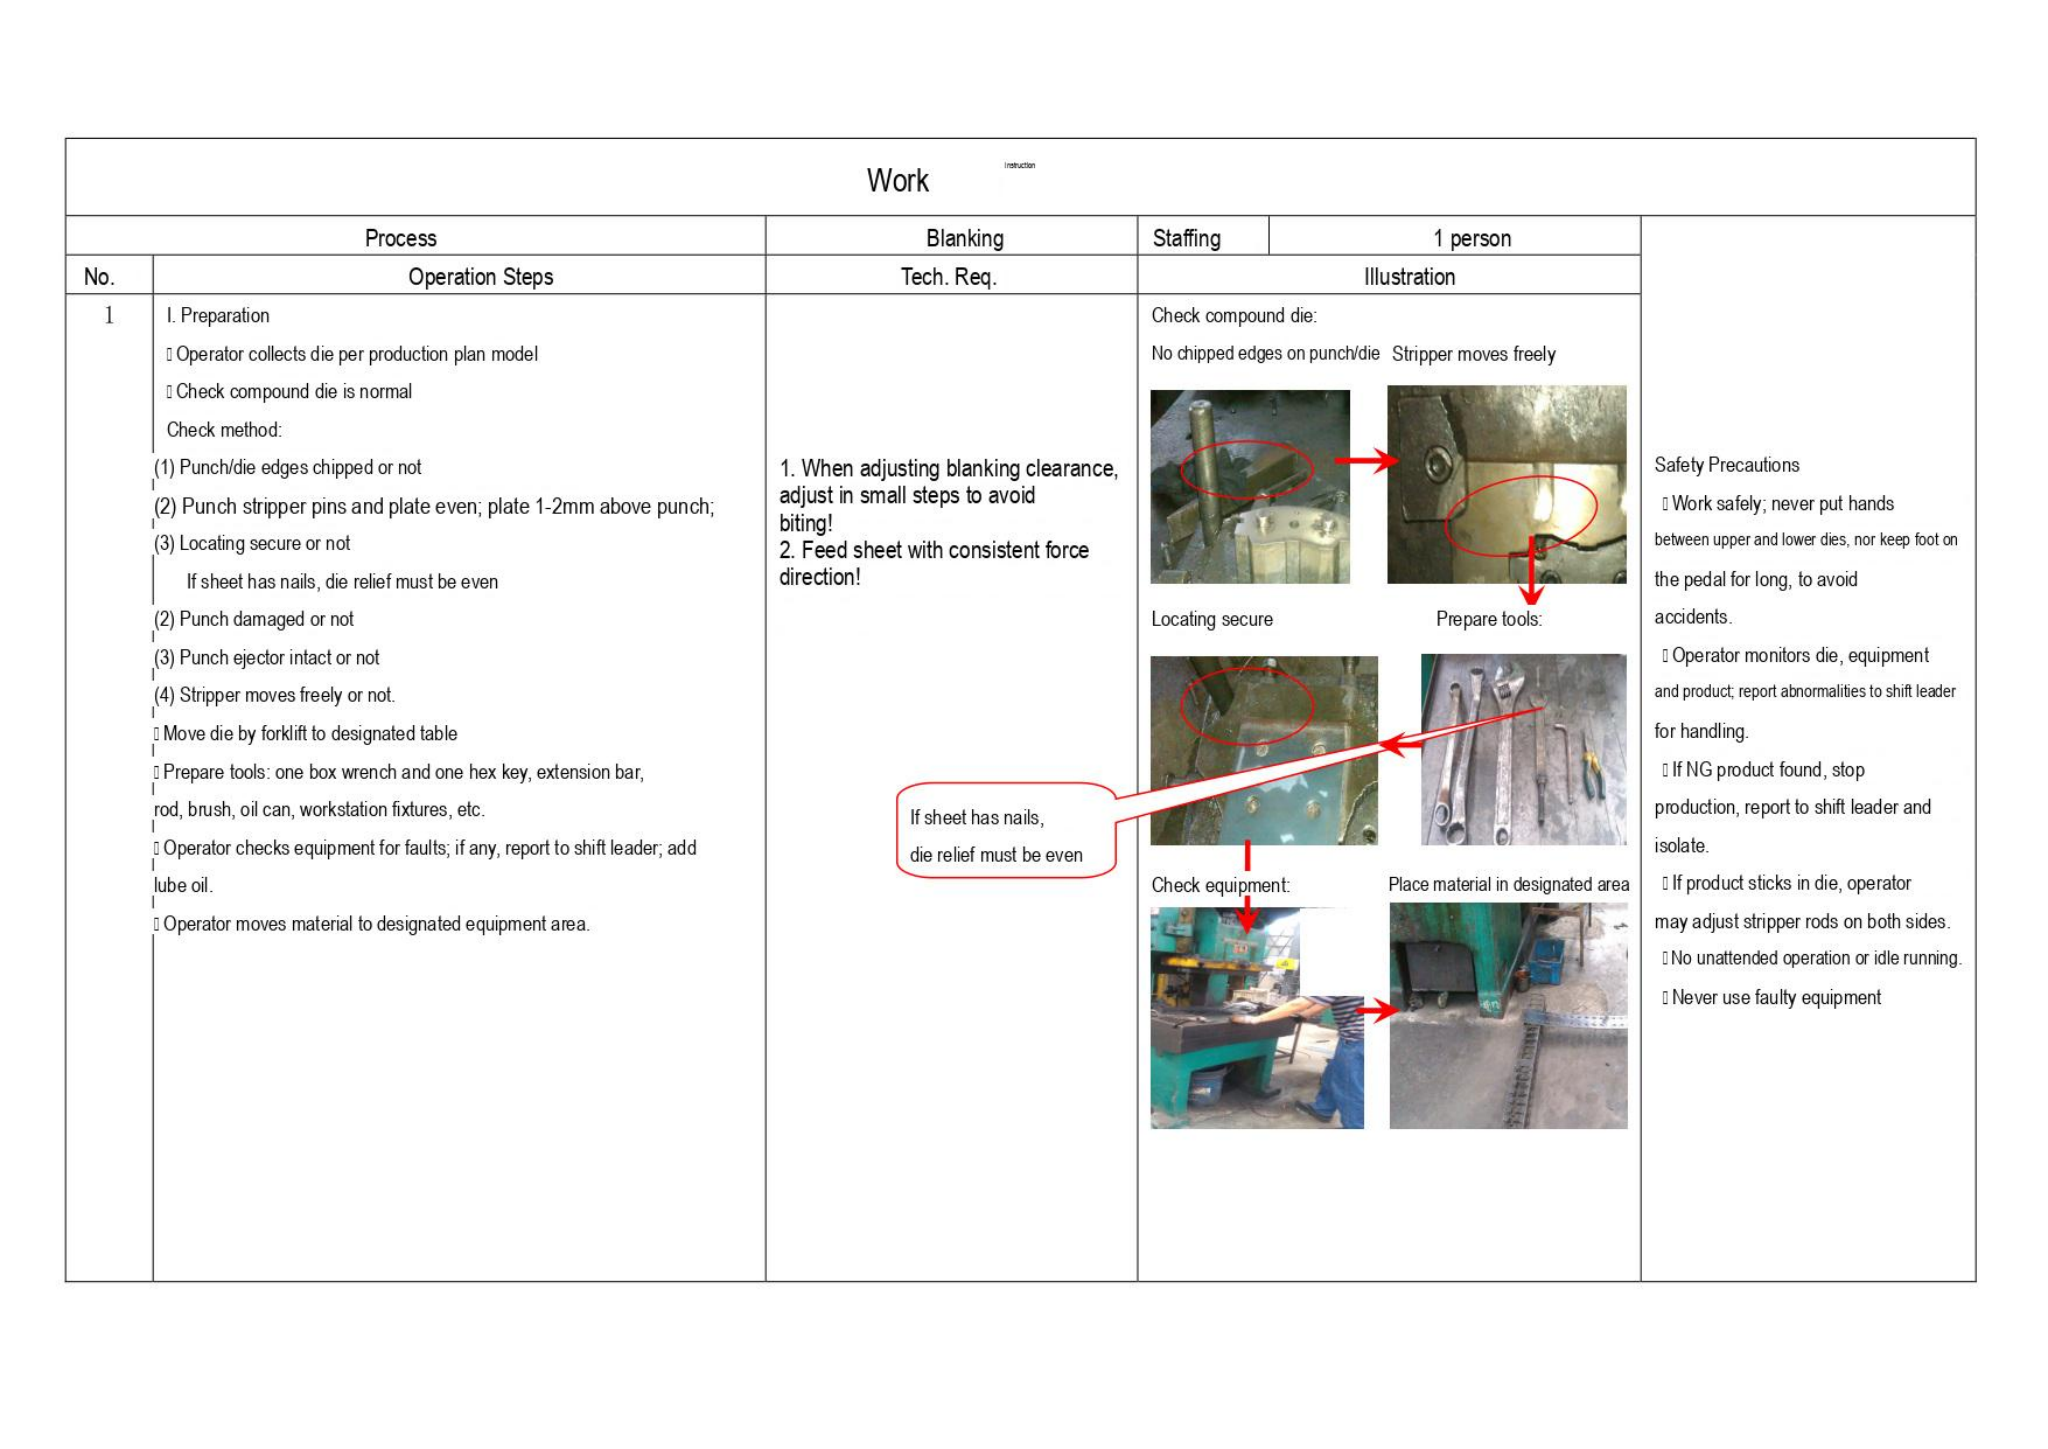# Work

Instruction

| Process | | Blanking | Staffing | 1 person | |
|---|---|---|---|---|---|
| **No.** | **Operation Steps** | **Tech. Req.** | **Illustration** | | |
| 1 | I. Preparation<br>Operator collects die per production plan model<br>Check compound die is normal<br>Check method:<br>(1) Punch/die edges chipped or not<br>(2) Punch stripper pins and plate even; plate 1-2mm above punch;<br>(3) Locating secure or not<br>If sheet has nails, die relief must be even<br>(2) Punch damaged or not<br>(3) Punch ejector intact or not<br>(4) Stripper moves freely or not.<br>Move die by forklift to designated table<br>Prepare tools: one box wrench and one hex key, extension bar, rod, brush, oil can, workstation fixtures, etc.<br>Operator checks equipment for faults; if any, report to shift leader; add lube oil.<br>Operator moves material to designated equipment area. | 1. When adjusting blanking clearance, adjust in small steps to avoid biting!<br>2. Feed sheet with consistent force direction!<br><br>If sheet has nails,<br>die relief must be even | Check compound die:<br>No chipped edges on punch/die<br>Stripper moves freely<br>Locating secure<br>Prepare tools:<br>Check equipment:<br>Place material in designated area | | Safety Precautions<br>Work safely; never put hands between upper and lower dies, nor keep foot on the pedal for long, to avoid accidents.<br>Operator monitors die, equipment and product; report abnormalities to shift leader for handling.<br>If NG product found, stop production, report to shift leader and isolate.<br>If product sticks in die, operator may adjust stripper rods on both sides.<br>No unattended operation or idle running.<br>Never use faulty equipment |
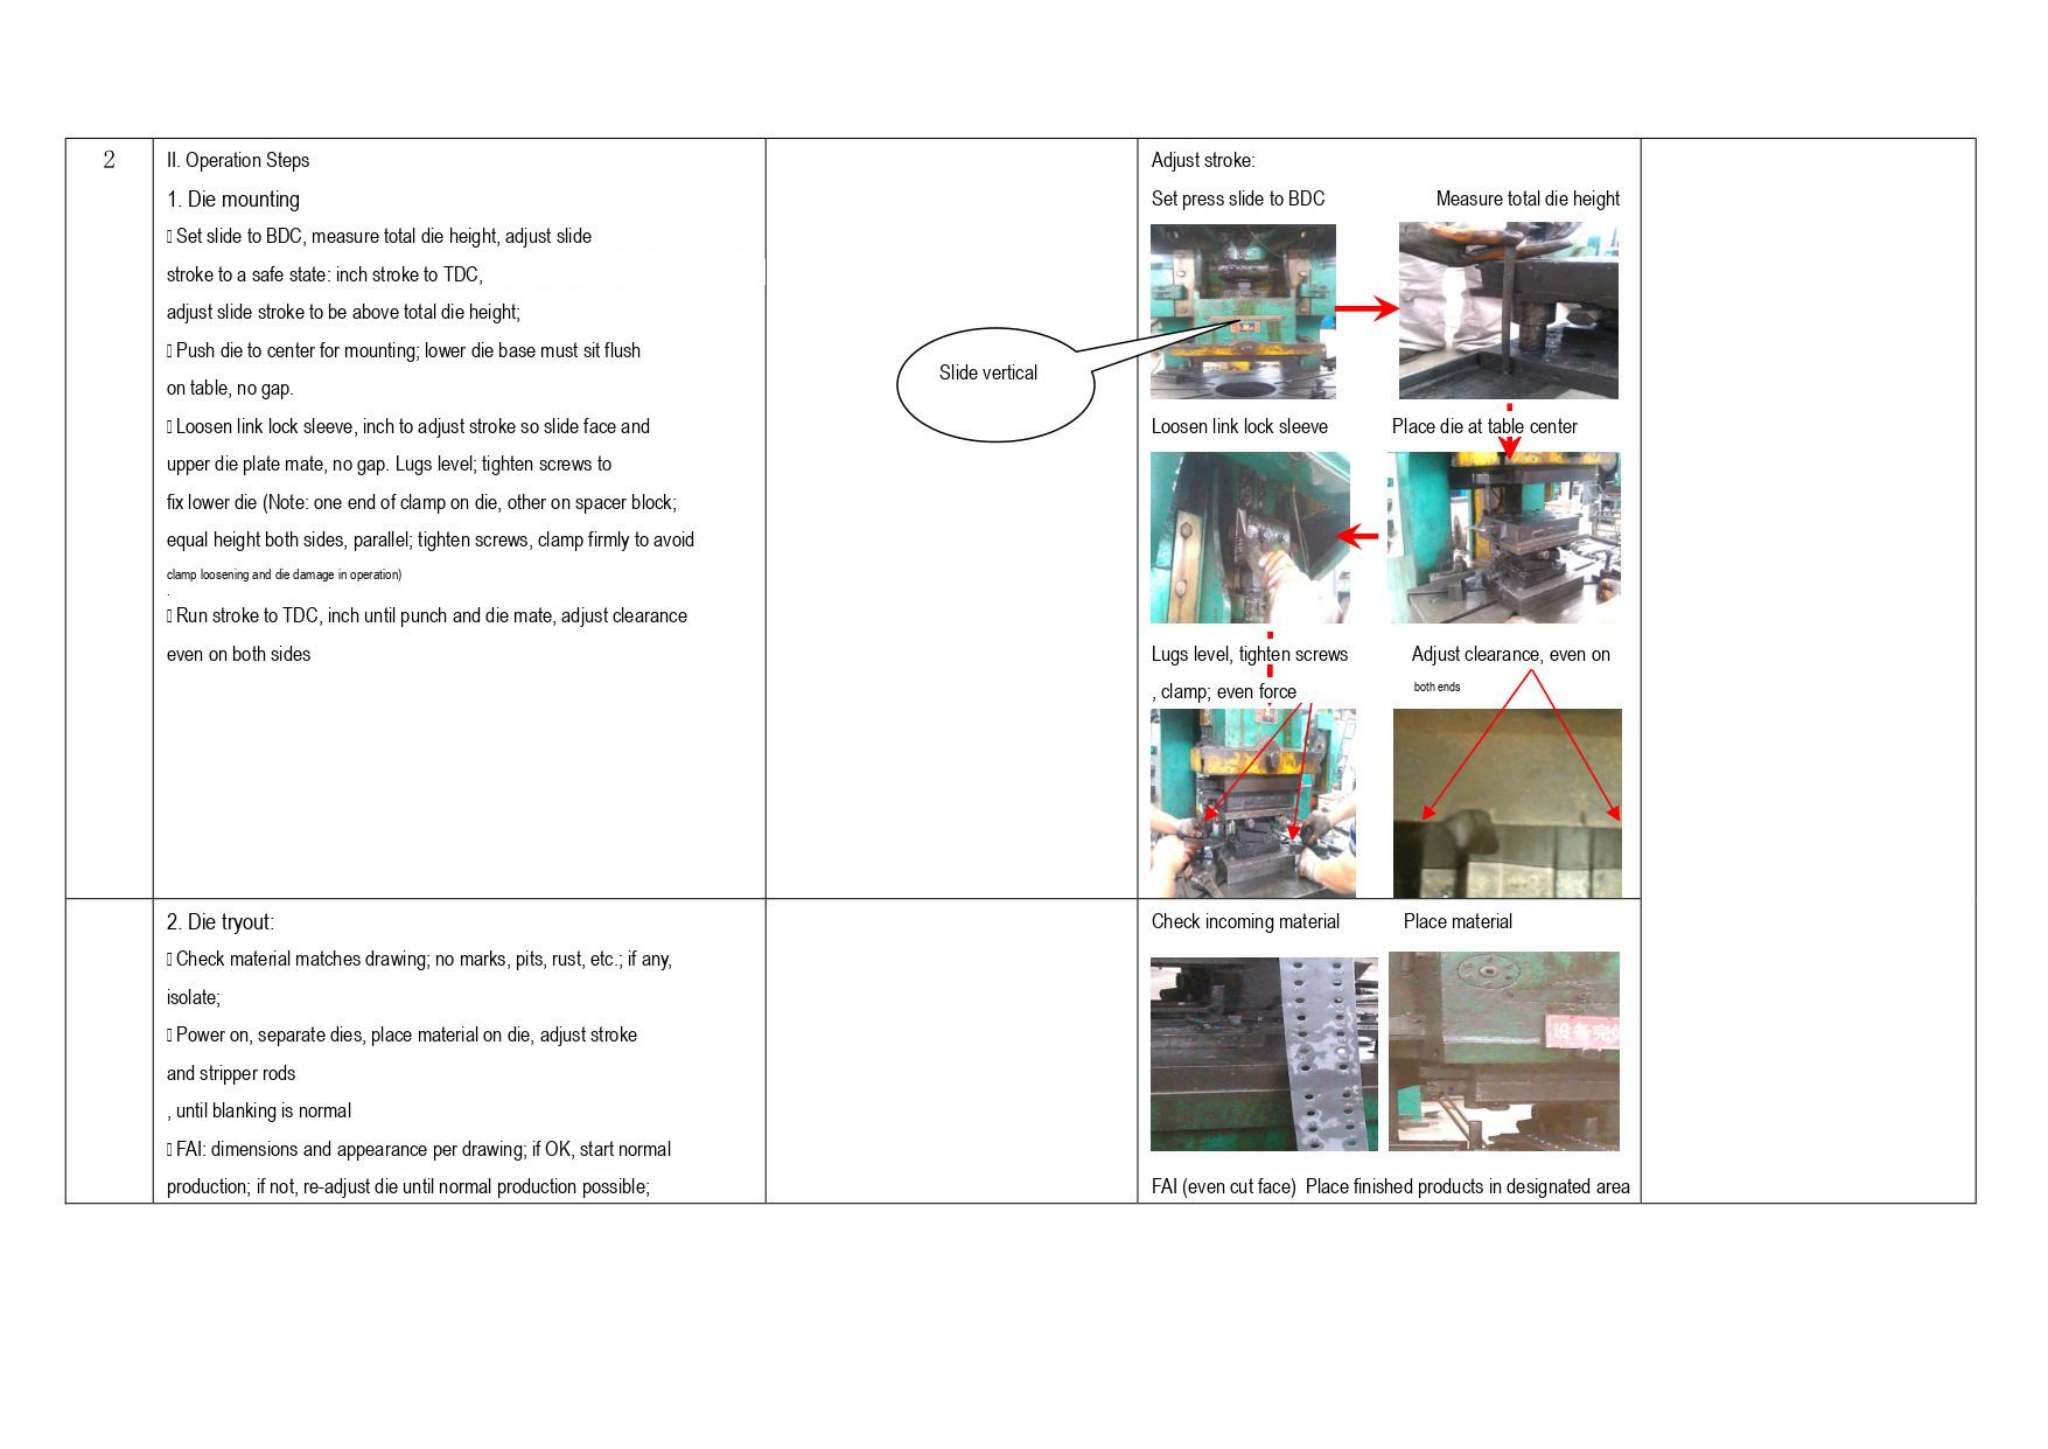| | | | | |
|---|---|---|---|---|
| 2 | II. Operation Steps<br>1. Die mounting<br>▯ Set slide to BDC, measure total die height, adjust slide stroke to a safe state: inch stroke to TDC, adjust slide stroke to be above total die height;<br>▯ Push die to center for mounting; lower die base must sit flush on table, no gap.<br>▯ Loosen link lock sleeve, inch to adjust stroke so slide face and upper die plate mate, no gap. Lugs level; tighten screws to fix lower die (Note: one end of clamp on die, other on spacer block; equal height both sides, parallel; tighten screws, clamp firmly to avoid clamp loosening and die damage in operation)<br>▯ Run stroke to TDC, inch until punch and die mate, adjust clearance even on both sides | Slide vertical | Adjust stroke:<br>Set press slide to BDC<br>Measure total die height<br>Loosen link lock sleeve<br>Place die at table center<br>Lugs level, tighten screws , clamp; even force<br>Adjust clearance, even on both ends | |
| | 2. Die tryout:<br>▯ Check material matches drawing; no marks, pits, rust, etc.; if any, isolate;<br>▯ Power on, separate dies, place material on die, adjust stroke and stripper rods , until blanking is normal<br>▯ FAI: dimensions and appearance per drawing; if OK, start normal production; if not, re-adjust die until normal production possible; | | Check incoming material<br>Place material<br>FAI (even cut face)<br>Place finished products in designated area | |
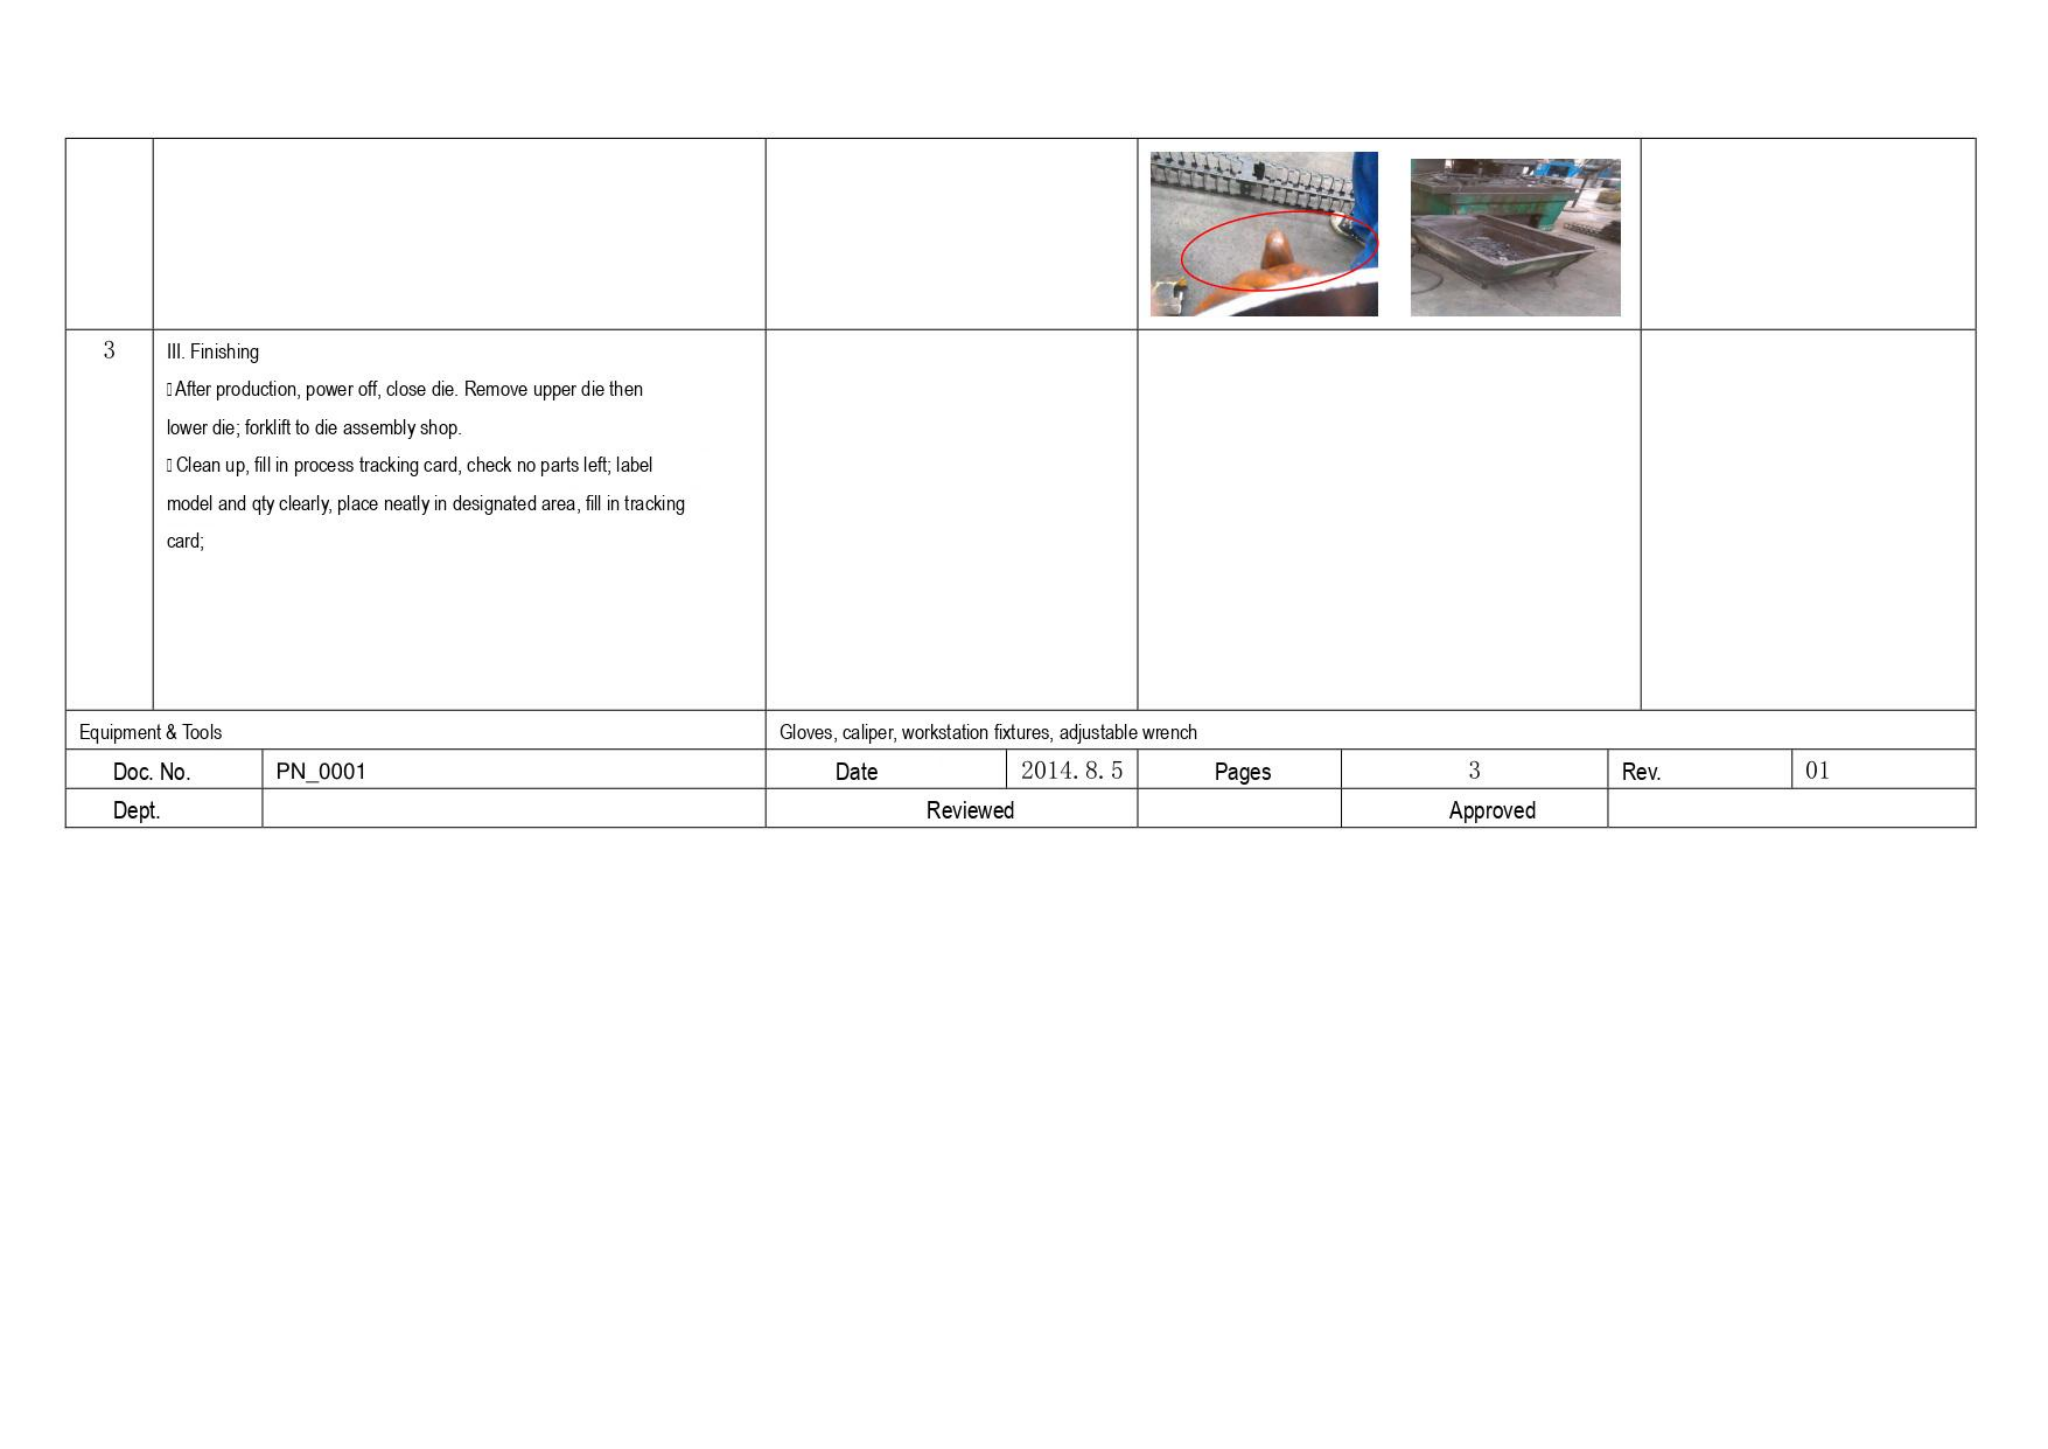|  |  |  |  |  |
|---|---|---|---|---|
|  |  |  |  |  |
| 3 | III. Finishing<br>After production, power off, close die. Remove upper die then lower die; forklift to die assembly shop.<br>Clean up, fill in process tracking card, check no parts left; label model and qty clearly, place neatly in designated area, fill in tracking card; |  |  |  |

| Equipment & Tools | Gloves, caliper, workstation fixtures, adjustable wrench |  |  |  |  |  |  |
|---|---|---|---|---|---|---|---|
| Doc. No. | PN_0001 | Date | 2014. 8. 5 | Pages | 3 | Rev. | 01 |
| Dept. |  | Reviewed |  | Approved |  |  |  |